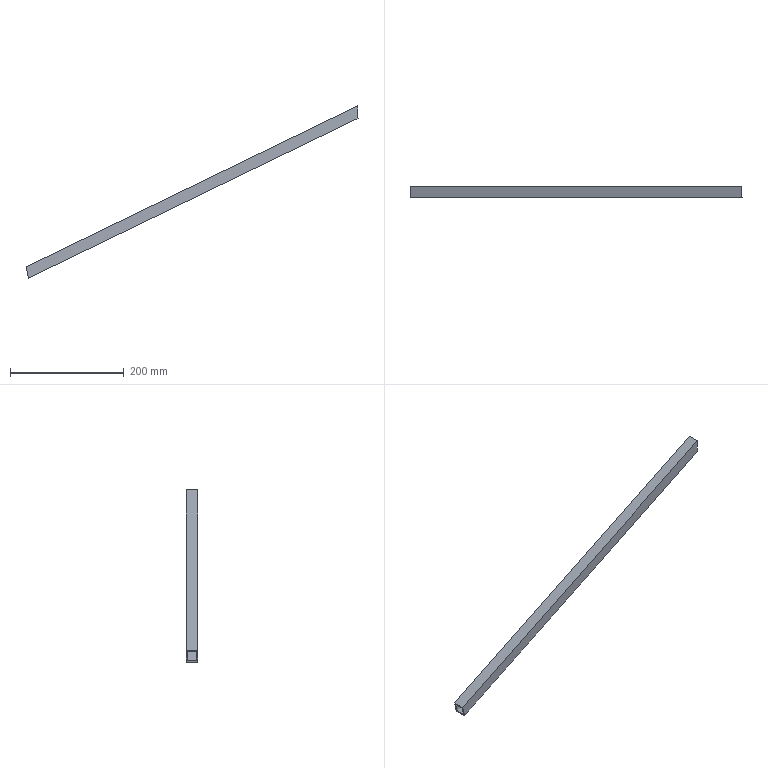Part | NX | features BREP 1 | 1 solid | 14 faces | volume 92693 mm3 | plane 10 | cylinder 4 | commonest cylinder face diameters 7 x4